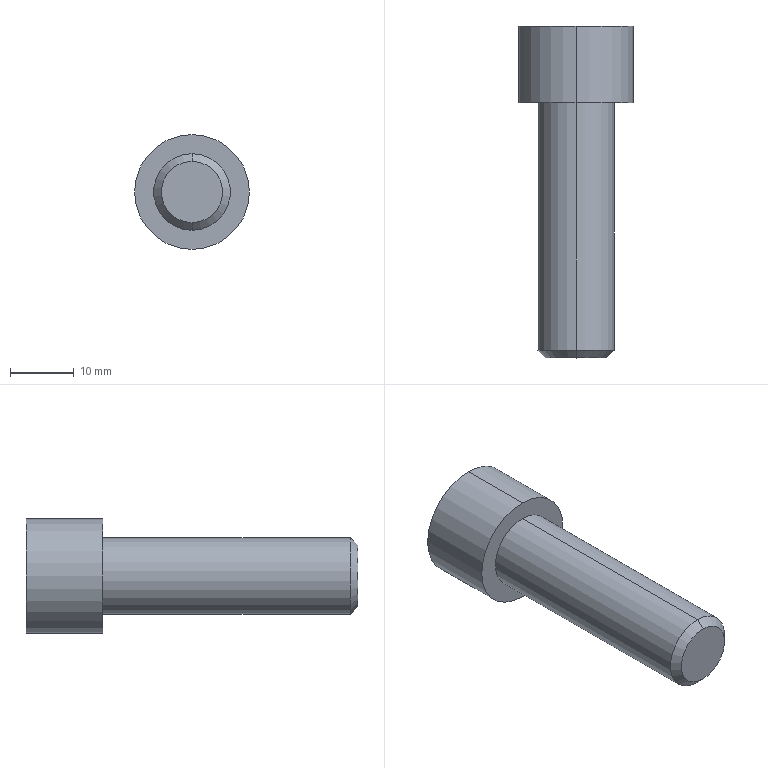Part | SolidWorks | features ICE 2, Chamfer 1, Extrusion 1, RevCut 1 | 1 solid | 29 faces | box 18 x 52 x 18 mm | volume 6970 mm3 | plane 15 | cone 10 | cylinder 4 | commonest cylinder face diameters 12 x2 18 x2
STEP:
#1=CARTESIAN_POINT('',(0.,-40.,-4.8));
#2=VERTEX_POINT('',#1);
#3=CARTESIAN_POINT('',(0.,-40.,4.8));
#4=VERTEX_POINT('',#3);
#5=CARTESIAN_POINT('',(0.,-40.,0.));
#6=DIRECTION('',(0.,-1.,0.));
#7=DIRECTION('',(0.,0.,-1.));
#8=AXIS2_PLACEMENT_3D('',#5,#6,#7);
#9=CIRCLE('',#8,4.8);
#10=EDGE_CURVE('',#2,#4,#9,.T.);
#11=ORIENTED_EDGE('',*,*,#10,.F.);
#12=CARTESIAN_POINT('',(0.,-38.8,-6.));
#13=VERTEX_POINT('',#12);
#14=CARTESIAN_POINT('',(0.,-40.,-4.8));
#15=DIRECTION('',(0.,0.7071,-0.7071));
#16=VECTOR('',#15,1000.);
#17=LINE('',#14,#16);
#18=EDGE_CURVE('',#2,#13,#17,.T.);
#19=ORIENTED_EDGE('',*,*,#18,.T.);
#20=CARTESIAN_POINT('',(0.,-38.8,6.));
#21=VERTEX_POINT('',#20);
#22=CARTESIAN_POINT('',(0.,-38.8,0.));
#23=DIRECTION('',(0.,1.,0.));
#24=DIRECTION('',(0.,0.,-1.));
#25=AXIS2_PLACEMENT_3D('',#22,#23,#24);
#26=CIRCLE('',#25,6.);
#27=EDGE_CURVE('',#21,#13,#26,.T.);
#28=ORIENTED_EDGE('',*,*,#27,.F.);
#29=CARTESIAN_POINT('',(0.,-40.,4.8));
#30=DIRECTION('',(0.,0.7071,0.7071));
#31=VECTOR('',#30,1000.);
#32=LINE('',#29,#31);
#33=EDGE_CURVE('',#4,#21,#32,.T.);
#34=ORIENTED_EDGE('',*,*,#33,.F.);
#35=EDGE_LOOP('',(#11,#19,#28,#34));
#36=FACE_OUTER_BOUND('',#35,.T.);
#37=CARTESIAN_POINT('',(0.,-40.,0.));
#38=DIRECTION('',(0.,1.,0.));
#39=DIRECTION('',(0.,0.,1.));
#40=AXIS2_PLACEMENT_3D('',#37,#38,#39);
#41=CONICAL_SURFACE('',#40,4.8,0.7854);
#42=ADVANCED_FACE('',(#36),#41,.T.);
#43=CARTESIAN_POINT('',(0.,3.15,0.));
#44=VERTEX_POINT('',#43);
#45=CARTESIAN_POINT('',(0.,6.,4.936));
#46=VERTEX_POINT('',#45);
#47=CARTESIAN_POINT('',(0.,3.15,0.));
#48=DIRECTION('',(0.,0.5,0.866));
#49=VECTOR('',#48,1000.);
#50=LINE('',#47,#49);
#51=EDGE_CURVE('',#44,#46,#50,.T.);
#52=ORIENTED_EDGE('',*,*,#51,.F.);
#53=CARTESIAN_POINT('',(0.,6.,-4.936));
#54=VERTEX_POINT('',#53);
#55=CARTESIAN_POINT('',(0.,3.15,0.));
#56=DIRECTION('',(0.,0.5,-0.866));
#57=VECTOR('',#56,1000.);
#58=LINE('',#55,#57);
#59=EDGE_CURVE('',#44,#54,#58,.T.);
#60=ORIENTED_EDGE('',*,*,#59,.T.);
#61=CARTESIAN_POINT('',(-2.468,6.,-4.275));
#62=VERTEX_POINT('',#61);
#63=CARTESIAN_POINT('',(0.,6.,0.));
#64=DIRECTION('',(0.,-1.,0.));
#65=DIRECTION('',(0.,0.,-1.));
#66=AXIS2_PLACEMENT_3D('',#63,#64,#65);
#67=CIRCLE('',#66,4.936);
#68=EDGE_CURVE('',#62,#54,#67,.T.);
#69=ORIENTED_EDGE('',*,*,#68,.F.);
#70=CARTESIAN_POINT('',(-4.936,6.,0.));
#71=VERTEX_POINT('',#70);
#72=CARTESIAN_POINT('',(0.,6.,0.));
#73=DIRECTION('',(0.,-1.,0.));
#74=DIRECTION('',(0.,0.,-1.));
#75=AXIS2_PLACEMENT_3D('',#72,#73,#74);
#76=CIRCLE('',#75,4.936);
#77=EDGE_CURVE('',#71,#62,#76,.T.);
#78=ORIENTED_EDGE('',*,*,#77,.F.);
#79=CARTESIAN_POINT('',(-2.468,6.,4.275));
#80=VERTEX_POINT('',#79);
#81=CARTESIAN_POINT('',(0.,6.,0.));
#82=DIRECTION('',(0.,-1.,0.));
#83=DIRECTION('',(0.,0.,-1.));
#84=AXIS2_PLACEMENT_3D('',#81,#82,#83);
#85=CIRCLE('',#84,4.936);
#86=EDGE_CURVE('',#80,#71,#85,.T.);
#87=ORIENTED_EDGE('',*,*,#86,.F.);
#88=CARTESIAN_POINT('',(0.,6.,0.));
#89=DIRECTION('',(0.,-1.,0.));
#90=DIRECTION('',(0.,0.,-1.));
#91=AXIS2_PLACEMENT_3D('',#88,#89,#90);
#92=CIRCLE('',#91,4.936);
#93=EDGE_CURVE('',#46,#80,#92,.T.);
#94=ORIENTED_EDGE('',*,*,#93,.F.);
#95=EDGE_LOOP('',(#52,#60,#69,#78,#87,#94));
#96=FACE_OUTER_BOUND('',#95,.T.);
#97=CARTESIAN_POINT('',(0.,1003.15,0.));
#98=DIRECTION('',(0.,1.,0.));
#99=DIRECTION('',(0.,0.,1.));
#100=AXIS2_PLACEMENT_3D('',#97,#98,#99);
#101=CONICAL_SURFACE('',#100,1732.051,1.047);
#102=ADVANCED_FACE('',(#96),#101,.F.);
#103=ORIENTED_EDGE('',*,*,#27,.T.);
#104=CARTESIAN_POINT('',(0.,0.,-6.));
#105=VERTEX_POINT('',#104);
#106=CARTESIAN_POINT('',(0.,-40.,-6.));
#107=DIRECTION('',(0.,1.,0.));
#108=VECTOR('',#107,1000.);
#109=LINE('',#106,#108);
#110=EDGE_CURVE('',#13,#105,#109,.T.);
#111=ORIENTED_EDGE('',*,*,#110,.T.);
#112=CARTESIAN_POINT('',(0.,0.,6.));
#113=VERTEX_POINT('',#112);
#114=CARTESIAN_POINT('',(0.,0.,0.));
#115=DIRECTION('',(0.,-1.,0.));
#116=DIRECTION('',(0.,0.,1.));
#117=AXIS2_PLACEMENT_3D('',#114,#115,#116);
#118=CIRCLE('',#117,6.);
#119=EDGE_CURVE('',#105,#113,#118,.T.);
#120=ORIENTED_EDGE('',*,*,#119,.T.);
#121=CARTESIAN_POINT('',(0.,-40.,6.));
#122=DIRECTION('',(0.,1.,0.));
#123=VECTOR('',#122,1000.);
#124=LINE('',#121,#123);
#125=EDGE_CURVE('',#21,#113,#124,.T.);
#126=ORIENTED_EDGE('',*,*,#125,.F.);
#127=EDGE_LOOP('',(#103,#111,#120,#126));
#128=FACE_OUTER_BOUND('',#127,.T.);
#129=CARTESIAN_POINT('',(0.,-40.,0.));
#130=DIRECTION('',(0.,1.,0.));
#131=DIRECTION('',(0.,0.,1.));
#132=AXIS2_PLACEMENT_3D('',#129,#130,#131);
#133=CYLINDRICAL_SURFACE('',#132,6.);
#134=ADVANCED_FACE('',(#128),#133,.T.);
#135=CARTESIAN_POINT('',(0.,12.,9.));
#136=VERTEX_POINT('',#135);
#137=CARTESIAN_POINT('',(0.,12.,-9.));
#138=VERTEX_POINT('',#137);
#139=CARTESIAN_POINT('',(0.,12.,0.));
#140=DIRECTION('',(0.,1.,0.));
#141=DIRECTION('',(0.,0.,1.));
#142=AXIS2_PLACEMENT_3D('',#139,#140,#141);
#143=CIRCLE('',#142,9.);
#144=EDGE_CURVE('',#136,#138,#143,.T.);
#145=ORIENTED_EDGE('',*,*,#144,.F.);
#146=CARTESIAN_POINT('',(0.,0.,9.));
#147=VERTEX_POINT('',#146);
#148=CARTESIAN_POINT('',(0.,12.,9.));
#149=DIRECTION('',(0.,-1.,0.));
#150=VECTOR('',#149,1000.);
#151=LINE('',#148,#150);
#152=EDGE_CURVE('',#136,#147,#151,.T.);
#153=ORIENTED_EDGE('',*,*,#152,.T.);
#154=CARTESIAN_POINT('',(0.,0.,-9.));
#155=VERTEX_POINT('',#154);
#156=CARTESIAN_POINT('',(0.,0.,0.));
#157=DIRECTION('',(0.,1.,0.));
#158=DIRECTION('',(0.,0.,1.));
#159=AXIS2_PLACEMENT_3D('',#156,#157,#158);
#160=CIRCLE('',#159,9.);
#161=EDGE_CURVE('',#147,#155,#160,.T.);
#162=ORIENTED_EDGE('',*,*,#161,.T.);
#163=CARTESIAN_POINT('',(0.,12.,-9.));
#164=DIRECTION('',(0.,-1.,0.));
#165=VECTOR('',#164,1000.);
#166=LINE('',#163,#165);
#167=EDGE_CURVE('',#138,#155,#166,.T.);
#168=ORIENTED_EDGE('',*,*,#167,.F.);
#169=EDGE_LOOP('',(#145,#153,#162,#168));
#170=FACE_OUTER_BOUND('',#169,.T.);
#171=CARTESIAN_POINT('',(0.,12.,0.));
#172=DIRECTION('',(0.,-1.,0.));
#173=DIRECTION('',(0.,0.,-1.));
#174=AXIS2_PLACEMENT_3D('',#171,#172,#173);
#175=CYLINDRICAL_SURFACE('',#174,9.);
#176=ADVANCED_FACE('',(#170),#175,.T.);
#177=CARTESIAN_POINT('',(0.,0.,0.));
#178=DIRECTION('',(0.,1.,0.));
#179=DIRECTION('',(0.,0.,1.));
#180=AXIS2_PLACEMENT_3D('',#177,#178,#179);
#181=CIRCLE('',#180,9.);
#182=EDGE_CURVE('',#155,#147,#181,.T.);
#183=ORIENTED_EDGE('',*,*,#182,.F.);
#184=ORIENTED_EDGE('',*,*,#161,.F.);
#185=EDGE_LOOP('',(#183,#184));
#186=FACE_OUTER_BOUND('',#185,.T.);
#187=CARTESIAN_POINT('',(0.,0.,0.));
#188=DIRECTION('',(0.,-1.,0.));
#189=DIRECTION('',(0.,0.,1.));
#190=AXIS2_PLACEMENT_3D('',#187,#188,#189);
#191=CIRCLE('',#190,6.);
#192=EDGE_CURVE('',#113,#105,#191,.T.);
#193=ORIENTED_EDGE('',*,*,#192,.F.);
#194=ORIENTED_EDGE('',*,*,#119,.F.);
#195=EDGE_LOOP('',(#193,#194));
#196=FACE_BOUND('',#195,.T.);
#197=CARTESIAN_POINT('',(0.,0.,0.));
#198=DIRECTION('',(0.,1.,0.));
#199=DIRECTION('',(0.,0.,1.));
#200=AXIS2_PLACEMENT_3D('',#197,#198,#199);
#201=PLANE('',#200);
#202=ADVANCED_FACE('',(#186,#196),#201,.F.);
#203=ORIENTED_EDGE('',*,*,#152,.F.);
#204=CARTESIAN_POINT('',(0.,12.,0.));
#205=DIRECTION('',(0.,1.,0.));
#206=DIRECTION('',(0.,0.,1.));
#207=AXIS2_PLACEMENT_3D('',#204,#205,#206);
#208=CIRCLE('',#207,9.);
#209=EDGE_CURVE('',#138,#136,#208,.T.);
#210=ORIENTED_EDGE('',*,*,#209,.F.);
#211=ORIENTED_EDGE('',*,*,#167,.T.);
#212=ORIENTED_EDGE('',*,*,#182,.T.);
#213=EDGE_LOOP('',(#203,#210,#211,#212));
#214=FACE_OUTER_BOUND('',#213,.T.);
#215=CARTESIAN_POINT('',(0.,12.,0.));
#216=DIRECTION('',(0.,-1.,0.));
#217=DIRECTION('',(0.,0.,-1.));
#218=AXIS2_PLACEMENT_3D('',#215,#216,#217);
#219=CYLINDRICAL_SURFACE('',#218,9.);
#220=ADVANCED_FACE('',(#214),#219,.T.);
#221=CARTESIAN_POINT('',(4.936,12.,2.85));
#222=VERTEX_POINT('',#221);
#223=CARTESIAN_POINT('',(0.,12.,5.7));
#224=VERTEX_POINT('',#223);
#225=CARTESIAN_POINT('',(0.,12.,0.));
#226=DIRECTION('',(0.,-1.,0.));
#227=DIRECTION('',(0.,0.,-1.));
#228=AXIS2_PLACEMENT_3D('',#225,#226,#227);
#229=CIRCLE('',#228,5.7);
#230=EDGE_CURVE('',#222,#224,#229,.T.);
#231=ORIENTED_EDGE('',*,*,#230,.T.);
#232=CARTESIAN_POINT('',(-4.936,12.,2.85));
#233=VERTEX_POINT('',#232);
#234=CARTESIAN_POINT('',(0.,12.,0.));
#235=DIRECTION('',(0.,-1.,0.));
#236=DIRECTION('',(0.,0.,-1.));
#237=AXIS2_PLACEMENT_3D('',#234,#235,#236);
#238=CIRCLE('',#237,5.7);
#239=EDGE_CURVE('',#224,#233,#238,.T.);
#240=ORIENTED_EDGE('',*,*,#239,.T.);
#241=CARTESIAN_POINT('',(-4.936,12.,-2.85));
#242=VERTEX_POINT('',#241);
#243=CARTESIAN_POINT('',(0.,12.,0.));
#244=DIRECTION('',(0.,-1.,0.));
#245=DIRECTION('',(0.,0.,-1.));
#246=AXIS2_PLACEMENT_3D('',#243,#244,#245);
#247=CIRCLE('',#246,5.7);
#248=EDGE_CURVE('',#233,#242,#247,.T.);
#249=ORIENTED_EDGE('',*,*,#248,.T.);
#250=CARTESIAN_POINT('',(0.,12.,-5.7));
#251=VERTEX_POINT('',#250);
#252=CARTESIAN_POINT('',(0.,12.,0.));
#253=DIRECTION('',(0.,-1.,0.));
#254=DIRECTION('',(0.,0.,-1.));
#255=AXIS2_PLACEMENT_3D('',#252,#253,#254);
#256=CIRCLE('',#255,5.7);
#257=EDGE_CURVE('',#242,#251,#256,.T.);
#258=ORIENTED_EDGE('',*,*,#257,.T.);
#259=CARTESIAN_POINT('',(4.936,12.,-2.85));
#260=VERTEX_POINT('',#259);
#261=CARTESIAN_POINT('',(0.,12.,0.));
#262=DIRECTION('',(0.,-1.,0.));
#263=DIRECTION('',(0.,0.,-1.));
#264=AXIS2_PLACEMENT_3D('',#261,#262,#263);
#265=CIRCLE('',#264,5.7);
#266=EDGE_CURVE('',#251,#260,#265,.T.);
#267=ORIENTED_EDGE('',*,*,#266,.T.);
#268=CARTESIAN_POINT('',(0.,12.,0.));
#269=DIRECTION('',(0.,-1.,0.));
#270=DIRECTION('',(0.,0.,-1.));
#271=AXIS2_PLACEMENT_3D('',#268,#269,#270);
#272=CIRCLE('',#271,5.7);
#273=EDGE_CURVE('',#260,#222,#272,.T.);
#274=ORIENTED_EDGE('',*,*,#273,.T.);
#275=EDGE_LOOP('',(#231,#240,#249,#258,#267,#274));
#276=FACE_BOUND('',#275,.T.);
#277=ORIENTED_EDGE('',*,*,#209,.T.);
#278=ORIENTED_EDGE('',*,*,#144,.T.);
#279=EDGE_LOOP('',(#277,#278));
#280=FACE_OUTER_BOUND('',#279,.T.);
#281=CARTESIAN_POINT('',(0.,12.,0.));
#282=DIRECTION('',(0.,1.,0.));
#283=DIRECTION('',(0.,0.,1.));
#284=AXIS2_PLACEMENT_3D('',#281,#282,#283);
#285=PLANE('',#284);
#286=ADVANCED_FACE('',(#276,#280),#285,.T.);
#287=ORIENTED_EDGE('',*,*,#110,.F.);
#288=CARTESIAN_POINT('',(0.,-38.8,0.));
#289=DIRECTION('',(0.,1.,0.));
#290=DIRECTION('',(0.,0.,-1.));
#291=AXIS2_PLACEMENT_3D('',#288,#289,#290);
#292=CIRCLE('',#291,6.);
#293=EDGE_CURVE('',#13,#21,#292,.T.);
#294=ORIENTED_EDGE('',*,*,#293,.T.);
#295=ORIENTED_EDGE('',*,*,#125,.T.);
#296=ORIENTED_EDGE('',*,*,#192,.T.);
#297=EDGE_LOOP('',(#287,#294,#295,#296));
#298=FACE_OUTER_BOUND('',#297,.T.);
#299=CARTESIAN_POINT('',(0.,-40.,0.));
#300=DIRECTION('',(0.,1.,0.));
#301=DIRECTION('',(0.,0.,1.));
#302=AXIS2_PLACEMENT_3D('',#299,#300,#301);
#303=CYLINDRICAL_SURFACE('',#302,6.);
#304=ADVANCED_FACE('',(#298),#303,.T.);
#305=CARTESIAN_POINT('',(0.,-40.,0.));
#306=DIRECTION('',(0.,-1.,0.));
#307=DIRECTION('',(0.,0.,-1.));
#308=AXIS2_PLACEMENT_3D('',#305,#306,#307);
#309=CIRCLE('',#308,4.8);
#310=EDGE_CURVE('',#4,#2,#309,.T.);
#311=ORIENTED_EDGE('',*,*,#310,.T.);
#312=ORIENTED_EDGE('',*,*,#10,.T.);
#313=EDGE_LOOP('',(#311,#312));
#314=FACE_OUTER_BOUND('',#313,.T.);
#315=CARTESIAN_POINT('',(0.,-40.,0.));
#316=DIRECTION('',(0.,-1.,0.));
#317=DIRECTION('',(0.,0.,-1.));
#318=AXIS2_PLACEMENT_3D('',#315,#316,#317);
#319=PLANE('',#318);
#320=ADVANCED_FACE('',(#314),#319,.T.);
#321=ORIENTED_EDGE('',*,*,#257,.F.);
#322=CARTESIAN_POINT('',(0.,12.,-5.7));
#323=CARTESIAN_POINT('',(-0.806,11.731,-5.235));
#324=CARTESIAN_POINT('',(-1.624,11.56,-4.762));
#325=CARTESIAN_POINT('',(-2.673,11.559,-4.157));
#326=CARTESIAN_POINT('',(-2.884,11.569,-4.035));
#327=CARTESIAN_POINT('',(-3.301,11.609,-3.794));
#328=CARTESIAN_POINT('',(-3.508,11.639,-3.674));
#329=CARTESIAN_POINT('',(-4.126,11.755,-3.318));
#330=CARTESIAN_POINT('',(-4.533,11.865,-3.083));
#331=CARTESIAN_POINT('',(-4.936,12.,-2.85));
#332=B_SPLINE_CURVE_WITH_KNOTS('',3,(#322,#323,#324,#325,#326,#327,#328,#329,#330,#331),.UNSPECIFIED.,.F.,.F.,(4,2,2,2,4),(0.000000238,0.002879,0.003598,0.004318,0.005757),.UNSPECIFIED.);
#333=EDGE_CURVE('',#251,#242,#332,.T.);
#334=ORIENTED_EDGE('',*,*,#333,.F.);
#335=EDGE_LOOP('',(#321,#334));
#336=FACE_OUTER_BOUND('',#335,.T.);
#337=CARTESIAN_POINT('',(0.,11.559,0.));
#338=DIRECTION('',(0.,1.,0.));
#339=DIRECTION('',(0.,0.,1.));
#340=AXIS2_PLACEMENT_3D('',#337,#338,#339);
#341=CONICAL_SURFACE('',#340,4.936,1.047);
#342=ADVANCED_FACE('',(#336),#341,.F.);
#343=CARTESIAN_POINT('',(-4.936,12.,-2.85));
#344=CARTESIAN_POINT('',(-4.936,11.866,-2.386));
#345=CARTESIAN_POINT('',(-4.936,11.754,-1.911));
#346=CARTESIAN_POINT('',(-4.936,11.6,-0.9595));
#347=CARTESIAN_POINT('',(-4.936,11.559,-0.4809));
#348=CARTESIAN_POINT('',(-4.936,11.559,0.4826));
#349=CARTESIAN_POINT('',(-4.936,11.602,0.9709));
#350=CARTESIAN_POINT('',(-4.936,11.756,1.923));
#351=CARTESIAN_POINT('',(-4.936,11.867,2.389));
#352=CARTESIAN_POINT('',(-4.936,12.,2.85));
#353=B_SPLINE_CURVE_WITH_KNOTS('',3,(#343,#344,#345,#346,#347,#348,#349,#350,#351,#352),.UNSPECIFIED.,.F.,.F.,(4,2,2,2,4),(0.005085,0.006527,0.007969,0.009411,0.01085),.UNSPECIFIED.);
#354=EDGE_CURVE('',#242,#233,#353,.T.);
#355=ORIENTED_EDGE('',*,*,#354,.F.);
#356=ORIENTED_EDGE('',*,*,#248,.F.);
#357=EDGE_LOOP('',(#355,#356));
#358=FACE_OUTER_BOUND('',#357,.T.);
#359=CARTESIAN_POINT('',(0.,11.559,0.));
#360=DIRECTION('',(0.,1.,0.));
#361=DIRECTION('',(0.,0.,1.));
#362=AXIS2_PLACEMENT_3D('',#359,#360,#361);
#363=CONICAL_SURFACE('',#362,4.936,1.047);
#364=ADVANCED_FACE('',(#358),#363,.F.);
#365=CARTESIAN_POINT('',(-4.936,12.,2.85));
#366=CARTESIAN_POINT('',(-4.13,11.731,3.315));
#367=CARTESIAN_POINT('',(-3.312,11.56,3.788));
#368=CARTESIAN_POINT('',(-2.263,11.559,4.393));
#369=CARTESIAN_POINT('',(-2.052,11.569,4.515));
#370=CARTESIAN_POINT('',(-1.635,11.609,4.756));
#371=CARTESIAN_POINT('',(-1.428,11.639,4.876));
#372=CARTESIAN_POINT('',(-0.8104,11.755,5.232));
#373=CARTESIAN_POINT('',(-0.4035,11.865,5.467));
#374=CARTESIAN_POINT('',(0.,12.,5.7));
#375=B_SPLINE_CURVE_WITH_KNOTS('',3,(#365,#366,#367,#368,#369,#370,#371,#372,#373,#374),.UNSPECIFIED.,.F.,.F.,(4,2,2,2,4),(0.000000238,0.002879,0.003598,0.004318,0.005757),.UNSPECIFIED.);
#376=EDGE_CURVE('',#233,#224,#375,.T.);
#377=ORIENTED_EDGE('',*,*,#376,.F.);
#378=ORIENTED_EDGE('',*,*,#239,.F.);
#379=EDGE_LOOP('',(#377,#378));
#380=FACE_OUTER_BOUND('',#379,.T.);
#381=CARTESIAN_POINT('',(0.,11.559,0.));
#382=DIRECTION('',(0.,1.,0.));
#383=DIRECTION('',(0.,0.,1.));
#384=AXIS2_PLACEMENT_3D('',#381,#382,#383);
#385=CONICAL_SURFACE('',#384,4.936,1.047);
#386=ADVANCED_FACE('',(#380),#385,.F.);
#387=ORIENTED_EDGE('',*,*,#230,.F.);
#388=CARTESIAN_POINT('',(0.,12.,5.7));
#389=CARTESIAN_POINT('',(0.806,11.731,5.235));
#390=CARTESIAN_POINT('',(1.624,11.56,4.762));
#391=CARTESIAN_POINT('',(2.673,11.559,4.157));
#392=CARTESIAN_POINT('',(2.884,11.569,4.035));
#393=CARTESIAN_POINT('',(3.301,11.609,3.794));
#394=CARTESIAN_POINT('',(3.508,11.639,3.674));
#395=CARTESIAN_POINT('',(4.126,11.755,3.318));
#396=CARTESIAN_POINT('',(4.533,11.865,3.083));
#397=CARTESIAN_POINT('',(4.936,12.,2.85));
#398=B_SPLINE_CURVE_WITH_KNOTS('',3,(#388,#389,#390,#391,#392,#393,#394,#395,#396,#397),.UNSPECIFIED.,.F.,.F.,(4,2,2,2,4),(0.000000238,0.002879,0.003598,0.004318,0.005757),.UNSPECIFIED.);
#399=EDGE_CURVE('',#224,#222,#398,.T.);
#400=ORIENTED_EDGE('',*,*,#399,.F.);
#401=EDGE_LOOP('',(#387,#400));
#402=FACE_OUTER_BOUND('',#401,.T.);
#403=CARTESIAN_POINT('',(0.,11.559,0.));
#404=DIRECTION('',(0.,1.,0.));
#405=DIRECTION('',(0.,0.,1.));
#406=AXIS2_PLACEMENT_3D('',#403,#404,#405);
#407=CONICAL_SURFACE('',#406,4.936,1.047);
#408=ADVANCED_FACE('',(#402),#407,.F.);
#409=ORIENTED_EDGE('',*,*,#273,.F.);
#410=CARTESIAN_POINT('',(4.936,12.,2.85));
#411=CARTESIAN_POINT('',(4.936,11.867,2.389));
#412=CARTESIAN_POINT('',(4.936,11.756,1.923));
#413=CARTESIAN_POINT('',(4.936,11.602,0.9709));
#414=CARTESIAN_POINT('',(4.936,11.559,0.4826));
#415=CARTESIAN_POINT('',(4.936,11.559,-0.4809));
#416=CARTESIAN_POINT('',(4.936,11.6,-0.9595));
#417=CARTESIAN_POINT('',(4.936,11.754,-1.911));
#418=CARTESIAN_POINT('',(4.936,11.866,-2.386));
#419=CARTESIAN_POINT('',(4.936,12.,-2.85));
#420=B_SPLINE_CURVE_WITH_KNOTS('',3,(#410,#411,#412,#413,#414,#415,#416,#417,#418,#419),.UNSPECIFIED.,.F.,.F.,(4,2,2,2,4),(0.002089,0.003527,0.004966,0.006404,0.007842),.UNSPECIFIED.);
#421=EDGE_CURVE('',#222,#260,#420,.T.);
#422=ORIENTED_EDGE('',*,*,#421,.F.);
#423=EDGE_LOOP('',(#409,#422));
#424=FACE_OUTER_BOUND('',#423,.T.);
#425=CARTESIAN_POINT('',(0.,11.559,0.));
#426=DIRECTION('',(0.,1.,0.));
#427=DIRECTION('',(0.,0.,1.));
#428=AXIS2_PLACEMENT_3D('',#425,#426,#427);
#429=CONICAL_SURFACE('',#428,4.936,1.047);
#430=ADVANCED_FACE('',(#424),#429,.F.);
#431=ORIENTED_EDGE('',*,*,#266,.F.);
#432=CARTESIAN_POINT('',(4.936,12.,-2.85));
#433=CARTESIAN_POINT('',(4.13,11.731,-3.315));
#434=CARTESIAN_POINT('',(3.312,11.56,-3.788));
#435=CARTESIAN_POINT('',(2.263,11.559,-4.393));
#436=CARTESIAN_POINT('',(2.052,11.569,-4.515));
#437=CARTESIAN_POINT('',(1.635,11.609,-4.756));
#438=CARTESIAN_POINT('',(1.428,11.639,-4.876));
#439=CARTESIAN_POINT('',(0.8104,11.755,-5.232));
#440=CARTESIAN_POINT('',(0.4035,11.865,-5.467));
#441=CARTESIAN_POINT('',(0.,12.,-5.7));
#442=B_SPLINE_CURVE_WITH_KNOTS('',3,(#432,#433,#434,#435,#436,#437,#438,#439,#440,#441),.UNSPECIFIED.,.F.,.F.,(4,2,2,2,4),(0.000000238,0.002879,0.003598,0.004318,0.005757),.UNSPECIFIED.);
#443=EDGE_CURVE('',#260,#251,#442,.T.);
#444=ORIENTED_EDGE('',*,*,#443,.F.);
#445=EDGE_LOOP('',(#431,#444));
#446=FACE_OUTER_BOUND('',#445,.T.);
#447=CARTESIAN_POINT('',(0.,11.559,0.));
#448=DIRECTION('',(0.,1.,0.));
#449=DIRECTION('',(0.,0.,1.));
#450=AXIS2_PLACEMENT_3D('',#447,#448,#449);
#451=CONICAL_SURFACE('',#450,4.936,1.047);
#452=ADVANCED_FACE('',(#446),#451,.F.);
#453=ORIENTED_EDGE('',*,*,#59,.F.);
#454=ORIENTED_EDGE('',*,*,#51,.T.);
#455=CARTESIAN_POINT('',(2.468,6.,4.275));
#456=VERTEX_POINT('',#455);
#457=CARTESIAN_POINT('',(0.,6.,0.));
#458=DIRECTION('',(0.,-1.,0.));
#459=DIRECTION('',(0.,0.,-1.));
#460=AXIS2_PLACEMENT_3D('',#457,#458,#459);
#461=CIRCLE('',#460,4.936);
#462=EDGE_CURVE('',#456,#46,#461,.T.);
#463=ORIENTED_EDGE('',*,*,#462,.F.);
#464=CARTESIAN_POINT('',(4.936,6.,0.));
#465=VERTEX_POINT('',#464);
#466=CARTESIAN_POINT('',(0.,6.,0.));
#467=DIRECTION('',(0.,-1.,0.));
#468=DIRECTION('',(0.,0.,-1.));
#469=AXIS2_PLACEMENT_3D('',#466,#467,#468);
#470=CIRCLE('',#469,4.936);
#471=EDGE_CURVE('',#465,#456,#470,.T.);
#472=ORIENTED_EDGE('',*,*,#471,.F.);
#473=CARTESIAN_POINT('',(2.468,6.,-4.275));
#474=VERTEX_POINT('',#473);
#475=CARTESIAN_POINT('',(0.,6.,0.));
#476=DIRECTION('',(0.,-1.,0.));
#477=DIRECTION('',(0.,0.,-1.));
#478=AXIS2_PLACEMENT_3D('',#475,#476,#477);
#479=CIRCLE('',#478,4.936);
#480=EDGE_CURVE('',#474,#465,#479,.T.);
#481=ORIENTED_EDGE('',*,*,#480,.F.);
#482=CARTESIAN_POINT('',(0.,6.,0.));
#483=DIRECTION('',(0.,-1.,0.));
#484=DIRECTION('',(0.,0.,-1.));
#485=AXIS2_PLACEMENT_3D('',#482,#483,#484);
#486=CIRCLE('',#485,4.936);
#487=EDGE_CURVE('',#54,#474,#486,.T.);
#488=ORIENTED_EDGE('',*,*,#487,.F.);
#489=EDGE_LOOP('',(#453,#454,#463,#472,#481,#488));
#490=FACE_OUTER_BOUND('',#489,.T.);
#491=CARTESIAN_POINT('',(0.,1003.15,0.));
#492=DIRECTION('',(0.,1.,0.));
#493=DIRECTION('',(0.,0.,1.));
#494=AXIS2_PLACEMENT_3D('',#491,#492,#493);
#495=CONICAL_SURFACE('',#494,1732.051,1.047);
#496=ADVANCED_FACE('',(#490),#495,.F.);
#497=CARTESIAN_POINT('',(4.936,6.,-2.85));
#498=VERTEX_POINT('',#497);
#499=CARTESIAN_POINT('',(4.936,6.,-2.85));
#500=DIRECTION('',(-0.866,0.,-0.5));
#501=VECTOR('',#500,1000.);
#502=LINE('',#499,#501);
#503=EDGE_CURVE('',#498,#474,#502,.T.);
#504=ORIENTED_EDGE('',*,*,#503,.T.);
#505=ORIENTED_EDGE('',*,*,#480,.T.);
#506=CARTESIAN_POINT('',(4.936,6.,2.85));
#507=DIRECTION('',(0.,0.,-1.));
#508=VECTOR('',#507,1000.);
#509=LINE('',#506,#508);
#510=EDGE_CURVE('',#465,#498,#509,.T.);
#511=ORIENTED_EDGE('',*,*,#510,.T.);
#512=EDGE_LOOP('',(#504,#505,#511));
#513=FACE_OUTER_BOUND('',#512,.T.);
#514=CARTESIAN_POINT('',(0.,6.,0.));
#515=DIRECTION('',(0.,1.,0.));
#516=DIRECTION('',(0.,0.,1.));
#517=AXIS2_PLACEMENT_3D('',#514,#515,#516);
#518=PLANE('',#517);
#519=ADVANCED_FACE('',(#513),#518,.T.);
#520=CARTESIAN_POINT('',(4.936,6.,2.85));
#521=VERTEX_POINT('',#520);
#522=CARTESIAN_POINT('',(4.936,6.,2.85));
#523=DIRECTION('',(0.,0.,-1.));
#524=VECTOR('',#523,1000.);
#525=LINE('',#522,#524);
#526=EDGE_CURVE('',#521,#465,#525,.T.);
#527=ORIENTED_EDGE('',*,*,#526,.T.);
#528=ORIENTED_EDGE('',*,*,#471,.T.);
#529=CARTESIAN_POINT('',(0.,6.,5.7));
#530=DIRECTION('',(0.866,0.,-0.5));
#531=VECTOR('',#530,1000.);
#532=LINE('',#529,#531);
#533=EDGE_CURVE('',#456,#521,#532,.T.);
#534=ORIENTED_EDGE('',*,*,#533,.T.);
#535=EDGE_LOOP('',(#527,#528,#534));
#536=FACE_OUTER_BOUND('',#535,.T.);
#537=CARTESIAN_POINT('',(0.,6.,0.));
#538=DIRECTION('',(0.,1.,0.));
#539=DIRECTION('',(0.,0.,1.));
#540=AXIS2_PLACEMENT_3D('',#537,#538,#539);
#541=PLANE('',#540);
#542=ADVANCED_FACE('',(#536),#541,.T.);
#543=CARTESIAN_POINT('',(0.,6.,5.7));
#544=VERTEX_POINT('',#543);
#545=CARTESIAN_POINT('',(0.,6.,5.7));
#546=DIRECTION('',(0.866,0.,-0.5));
#547=VECTOR('',#546,1000.);
#548=LINE('',#545,#547);
#549=EDGE_CURVE('',#544,#456,#548,.T.);
#550=ORIENTED_EDGE('',*,*,#549,.T.);
#551=ORIENTED_EDGE('',*,*,#462,.T.);
#552=ORIENTED_EDGE('',*,*,#93,.T.);
#553=CARTESIAN_POINT('',(-4.936,6.,2.85));
#554=DIRECTION('',(0.866,0.,0.5));
#555=VECTOR('',#554,1000.);
#556=LINE('',#553,#555);
#557=EDGE_CURVE('',#80,#544,#556,.T.);
#558=ORIENTED_EDGE('',*,*,#557,.T.);
#559=EDGE_LOOP('',(#550,#551,#552,#558));
#560=FACE_OUTER_BOUND('',#559,.T.);
#561=CARTESIAN_POINT('',(0.,6.,0.));
#562=DIRECTION('',(0.,1.,0.));
#563=DIRECTION('',(0.,0.,1.));
#564=AXIS2_PLACEMENT_3D('',#561,#562,#563);
#565=PLANE('',#564);
#566=ADVANCED_FACE('',(#560),#565,.T.);
#567=CARTESIAN_POINT('',(-4.936,6.,2.85));
#568=VERTEX_POINT('',#567);
#569=CARTESIAN_POINT('',(-4.936,6.,2.85));
#570=DIRECTION('',(0.866,0.,0.5));
#571=VECTOR('',#570,1000.);
#572=LINE('',#569,#571);
#573=EDGE_CURVE('',#568,#80,#572,.T.);
#574=ORIENTED_EDGE('',*,*,#573,.T.);
#575=ORIENTED_EDGE('',*,*,#86,.T.);
#576=CARTESIAN_POINT('',(-4.936,6.,-2.85));
#577=DIRECTION('',(0.,0.,1.));
#578=VECTOR('',#577,1000.);
#579=LINE('',#576,#578);
#580=EDGE_CURVE('',#71,#568,#579,.T.);
#581=ORIENTED_EDGE('',*,*,#580,.T.);
#582=EDGE_LOOP('',(#574,#575,#581));
#583=FACE_OUTER_BOUND('',#582,.T.);
#584=CARTESIAN_POINT('',(0.,6.,0.));
#585=DIRECTION('',(0.,1.,0.));
#586=DIRECTION('',(0.,0.,1.));
#587=AXIS2_PLACEMENT_3D('',#584,#585,#586);
#588=PLANE('',#587);
#589=ADVANCED_FACE('',(#583),#588,.T.);
#590=CARTESIAN_POINT('',(0.,6.,-5.7));
#591=VERTEX_POINT('',#590);
#592=CARTESIAN_POINT('',(0.,6.,-5.7));
#593=DIRECTION('',(-0.866,0.,0.5));
#594=VECTOR('',#593,1000.);
#595=LINE('',#592,#594);
#596=EDGE_CURVE('',#591,#62,#595,.T.);
#597=ORIENTED_EDGE('',*,*,#596,.T.);
#598=ORIENTED_EDGE('',*,*,#68,.T.);
#599=ORIENTED_EDGE('',*,*,#487,.T.);
#600=CARTESIAN_POINT('',(4.936,6.,-2.85));
#601=DIRECTION('',(-0.866,0.,-0.5));
#602=VECTOR('',#601,1000.);
#603=LINE('',#600,#602);
#604=EDGE_CURVE('',#474,#591,#603,.T.);
#605=ORIENTED_EDGE('',*,*,#604,.T.);
#606=EDGE_LOOP('',(#597,#598,#599,#605));
#607=FACE_OUTER_BOUND('',#606,.T.);
#608=CARTESIAN_POINT('',(0.,6.,0.));
#609=DIRECTION('',(0.,1.,0.));
#610=DIRECTION('',(0.,0.,1.));
#611=AXIS2_PLACEMENT_3D('',#608,#609,#610);
#612=PLANE('',#611);
#613=ADVANCED_FACE('',(#607),#612,.T.);
#614=CARTESIAN_POINT('',(-4.936,6.,-2.85));
#615=VERTEX_POINT('',#614);
#616=CARTESIAN_POINT('',(-4.936,6.,-2.85));
#617=DIRECTION('',(0.,0.,1.));
#618=VECTOR('',#617,1000.);
#619=LINE('',#616,#618);
#620=EDGE_CURVE('',#615,#71,#619,.T.);
#621=ORIENTED_EDGE('',*,*,#620,.T.);
#622=ORIENTED_EDGE('',*,*,#77,.T.);
#623=CARTESIAN_POINT('',(0.,6.,-5.7));
#624=DIRECTION('',(-0.866,0.,0.5));
#625=VECTOR('',#624,1000.);
#626=LINE('',#623,#625);
#627=EDGE_CURVE('',#62,#615,#626,.T.);
#628=ORIENTED_EDGE('',*,*,#627,.T.);
#629=EDGE_LOOP('',(#621,#622,#628));
#630=FACE_OUTER_BOUND('',#629,.T.);
#631=CARTESIAN_POINT('',(0.,6.,0.));
#632=DIRECTION('',(0.,1.,0.));
#633=DIRECTION('',(0.,0.,1.));
#634=AXIS2_PLACEMENT_3D('',#631,#632,#633);
#635=PLANE('',#634);
#636=ADVANCED_FACE('',(#630),#635,.T.);
#637=CARTESIAN_POINT('',(0.,6.,-5.7));
#638=DIRECTION('',(0.,1.,0.));
#639=VECTOR('',#638,1000.);
#640=LINE('',#637,#639);
#641=EDGE_CURVE('',#591,#251,#640,.T.);
#642=ORIENTED_EDGE('',*,*,#641,.T.);
#643=ORIENTED_EDGE('',*,*,#333,.T.);
#644=CARTESIAN_POINT('',(-4.936,6.,-2.85));
#645=DIRECTION('',(0.,1.,0.));
#646=VECTOR('',#645,1000.);
#647=LINE('',#644,#646);
#648=EDGE_CURVE('',#615,#242,#647,.T.);
#649=ORIENTED_EDGE('',*,*,#648,.F.);
#650=ORIENTED_EDGE('',*,*,#627,.F.);
#651=ORIENTED_EDGE('',*,*,#596,.F.);
#652=EDGE_LOOP('',(#642,#643,#649,#650,#651));
#653=FACE_OUTER_BOUND('',#652,.T.);
#654=CARTESIAN_POINT('',(0.,6.,-5.7));
#655=DIRECTION('',(-0.5,0.,-0.866));
#656=DIRECTION('',(-0.866,0.,0.5));
#657=AXIS2_PLACEMENT_3D('',#654,#655,#656);
#658=PLANE('',#657);
#659=ADVANCED_FACE('',(#653),#658,.F.);
#660=ORIENTED_EDGE('',*,*,#648,.T.);
#661=ORIENTED_EDGE('',*,*,#354,.T.);
#662=CARTESIAN_POINT('',(-4.936,6.,2.85));
#663=DIRECTION('',(0.,1.,0.));
#664=VECTOR('',#663,1000.);
#665=LINE('',#662,#664);
#666=EDGE_CURVE('',#568,#233,#665,.T.);
#667=ORIENTED_EDGE('',*,*,#666,.F.);
#668=ORIENTED_EDGE('',*,*,#580,.F.);
#669=ORIENTED_EDGE('',*,*,#620,.F.);
#670=EDGE_LOOP('',(#660,#661,#667,#668,#669));
#671=FACE_OUTER_BOUND('',#670,.T.);
#672=CARTESIAN_POINT('',(-4.936,6.,-2.85));
#673=DIRECTION('',(-1.,0.,0.));
#674=DIRECTION('',(0.,0.,1.));
#675=AXIS2_PLACEMENT_3D('',#672,#673,#674);
#676=PLANE('',#675);
#677=ADVANCED_FACE('',(#671),#676,.F.);
#678=ORIENTED_EDGE('',*,*,#666,.T.);
#679=ORIENTED_EDGE('',*,*,#376,.T.);
#680=CARTESIAN_POINT('',(0.,6.,5.7));
#681=DIRECTION('',(0.,1.,0.));
#682=VECTOR('',#681,1000.);
#683=LINE('',#680,#682);
#684=EDGE_CURVE('',#544,#224,#683,.T.);
#685=ORIENTED_EDGE('',*,*,#684,.F.);
#686=ORIENTED_EDGE('',*,*,#557,.F.);
#687=ORIENTED_EDGE('',*,*,#573,.F.);
#688=EDGE_LOOP('',(#678,#679,#685,#686,#687));
#689=FACE_OUTER_BOUND('',#688,.T.);
#690=CARTESIAN_POINT('',(-4.936,6.,2.85));
#691=DIRECTION('',(-0.5,0.,0.866));
#692=DIRECTION('',(0.866,0.,0.5));
#693=AXIS2_PLACEMENT_3D('',#690,#691,#692);
#694=PLANE('',#693);
#695=ADVANCED_FACE('',(#689),#694,.F.);
#696=ORIENTED_EDGE('',*,*,#684,.T.);
#697=ORIENTED_EDGE('',*,*,#399,.T.);
#698=CARTESIAN_POINT('',(4.936,6.,2.85));
#699=DIRECTION('',(0.,1.,0.));
#700=VECTOR('',#699,1000.);
#701=LINE('',#698,#700);
#702=EDGE_CURVE('',#521,#222,#701,.T.);
#703=ORIENTED_EDGE('',*,*,#702,.F.);
#704=ORIENTED_EDGE('',*,*,#533,.F.);
#705=ORIENTED_EDGE('',*,*,#549,.F.);
#706=EDGE_LOOP('',(#696,#697,#703,#704,#705));
#707=FACE_OUTER_BOUND('',#706,.T.);
#708=CARTESIAN_POINT('',(0.,6.,5.7));
#709=DIRECTION('',(0.5,0.,0.866));
#710=DIRECTION('',(0.866,0.,-0.5));
#711=AXIS2_PLACEMENT_3D('',#708,#709,#710);
#712=PLANE('',#711);
#713=ADVANCED_FACE('',(#707),#712,.F.);
#714=ORIENTED_EDGE('',*,*,#702,.T.);
#715=ORIENTED_EDGE('',*,*,#421,.T.);
#716=CARTESIAN_POINT('',(4.936,6.,-2.85));
#717=DIRECTION('',(0.,1.,0.));
#718=VECTOR('',#717,1000.);
#719=LINE('',#716,#718);
#720=EDGE_CURVE('',#498,#260,#719,.T.);
#721=ORIENTED_EDGE('',*,*,#720,.F.);
#722=ORIENTED_EDGE('',*,*,#510,.F.);
#723=ORIENTED_EDGE('',*,*,#526,.F.);
#724=EDGE_LOOP('',(#714,#715,#721,#722,#723));
#725=FACE_OUTER_BOUND('',#724,.T.);
#726=CARTESIAN_POINT('',(4.936,6.,2.85));
#727=DIRECTION('',(1.,0.,0.));
#728=DIRECTION('',(0.,0.,-1.));
#729=AXIS2_PLACEMENT_3D('',#726,#727,#728);
#730=PLANE('',#729);
#731=ADVANCED_FACE('',(#725),#730,.F.);
#732=ORIENTED_EDGE('',*,*,#720,.T.);
#733=ORIENTED_EDGE('',*,*,#443,.T.);
#734=ORIENTED_EDGE('',*,*,#641,.F.);
#735=ORIENTED_EDGE('',*,*,#604,.F.);
#736=ORIENTED_EDGE('',*,*,#503,.F.);
#737=EDGE_LOOP('',(#732,#733,#734,#735,#736));
#738=FACE_OUTER_BOUND('',#737,.T.);
#739=CARTESIAN_POINT('',(4.936,6.,-2.85));
#740=DIRECTION('',(0.5,0.,-0.866));
#741=DIRECTION('',(-0.866,0.,-0.5));
#742=AXIS2_PLACEMENT_3D('',#739,#740,#741);
#743=PLANE('',#742);
#744=ADVANCED_FACE('',(#738),#743,.F.);
#745=ORIENTED_EDGE('',*,*,#18,.F.);
#746=ORIENTED_EDGE('',*,*,#310,.F.);
#747=ORIENTED_EDGE('',*,*,#33,.T.);
#748=ORIENTED_EDGE('',*,*,#293,.F.);
#749=EDGE_LOOP('',(#745,#746,#747,#748));
#750=FACE_OUTER_BOUND('',#749,.T.);
#751=CARTESIAN_POINT('',(0.,-40.,0.));
#752=DIRECTION('',(0.,1.,0.));
#753=DIRECTION('',(0.,0.,1.));
#754=AXIS2_PLACEMENT_3D('',#751,#752,#753);
#755=CONICAL_SURFACE('',#754,4.8,0.7854);
#756=ADVANCED_FACE('',(#750),#755,.T.);
#757=CLOSED_SHELL('',(#42,#102,#134,#176,#202,#220,#286,#304,#320,#342,#364,#386,#408,#430,#452,#496,#519,#542,#566,#589,#613,#636,#659,#677,#695,#713,#731,#744,#756));
#758=MANIFOLD_SOLID_BREP('',#757);
#759=CARTESIAN_POINT('',(0.,0.,0.));
#760=DIRECTION('',(0.,0.,1.));
#761=DIRECTION('',(1.,0.,0.));
#762=AXIS2_PLACEMENT_3D('',#759,#760,#761);
#763=(LENGTH_UNIT()NAMED_UNIT(*)SI_UNIT(.MILLI.,.METRE.));
#764=UNCERTAINTY_MEASURE_WITH_UNIT(LENGTH_MEASURE(0.00001),#763,'','');
#765=(NAMED_UNIT(*)PLANE_ANGLE_UNIT()SI_UNIT($,.RADIAN.));
#766=(NAMED_UNIT(*)SI_UNIT($,.STERADIAN.)SOLID_ANGLE_UNIT());
#767=(GEOMETRIC_REPRESENTATION_CONTEXT(3)GLOBAL_UNCERTAINTY_ASSIGNED_CONTEXT((#764))GLOBAL_UNIT_ASSIGNED_CONTEXT((#763,#765,#766))REPRESENTATION_CONTEXT('',''));
#768=ADVANCED_BREP_SHAPE_REPRESENTATION('',(#758,#762),#767);